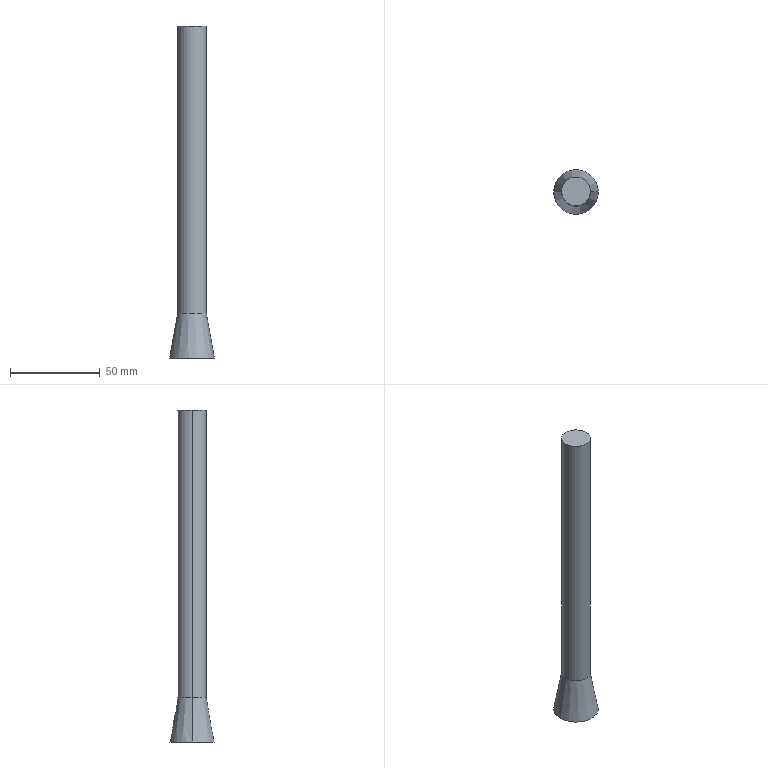Part | STEP file | part 159^COMPANY_A 408 evaporator | 1 solid | 36 faces | box 24.816 x 24.816 x 185 mm | volume 40377 mm3 | cylinder 22 | plane 12 | cone 2 | commonest cylinder face diameters 5 x20 16 x2